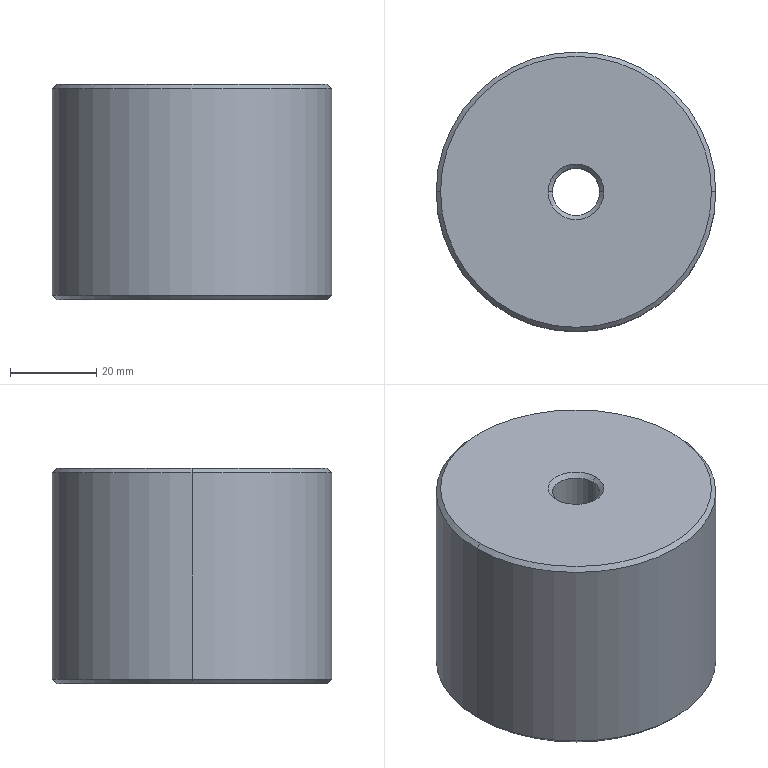Part | SolidWorks | features Chamfer 1, Extrusion 1 | 1 solid | 14 faces | box 65 x 65 x 50 mm | volume 160925 mm3 | cone 8 | cylinder 4 | plane 2 | commonest cylinder face diameters 11 x2 65 x2
STEP:
#1=CARTESIAN_POINT('',(31.5,0.,50.));
#2=VERTEX_POINT('',#1);
#3=CARTESIAN_POINT('',(-31.5,0.,50.));
#4=VERTEX_POINT('',#3);
#5=CARTESIAN_POINT('',(0.,0.,50.));
#6=DIRECTION('',(0.,0.,1.));
#7=DIRECTION('',(1.,0.,0.));
#8=AXIS2_PLACEMENT_3D('',#5,#6,#7);
#9=CIRCLE('',#8,31.5);
#10=EDGE_CURVE('',#2,#4,#9,.T.);
#11=ORIENTED_EDGE('',*,*,#10,.F.);
#12=CARTESIAN_POINT('',(32.5,0.,49.));
#13=VERTEX_POINT('',#12);
#14=CARTESIAN_POINT('',(31.5,0.,50.));
#15=DIRECTION('',(0.7071,0.,-0.7071));
#16=VECTOR('',#15,1000.);
#17=LINE('',#14,#16);
#18=EDGE_CURVE('',#2,#13,#17,.T.);
#19=ORIENTED_EDGE('',*,*,#18,.T.);
#20=CARTESIAN_POINT('',(-32.5,0.,49.));
#21=VERTEX_POINT('',#20);
#22=CARTESIAN_POINT('',(0.,0.,49.));
#23=DIRECTION('',(0.,0.,-1.));
#24=DIRECTION('',(1.,0.,0.));
#25=AXIS2_PLACEMENT_3D('',#22,#23,#24);
#26=CIRCLE('',#25,32.5);
#27=EDGE_CURVE('',#21,#13,#26,.T.);
#28=ORIENTED_EDGE('',*,*,#27,.F.);
#29=CARTESIAN_POINT('',(-31.5,0.,50.));
#30=DIRECTION('',(-0.7071,0.,-0.7071));
#31=VECTOR('',#30,1000.);
#32=LINE('',#29,#31);
#33=EDGE_CURVE('',#4,#21,#32,.T.);
#34=ORIENTED_EDGE('',*,*,#33,.F.);
#35=EDGE_LOOP('',(#11,#19,#28,#34));
#36=FACE_OUTER_BOUND('',#35,.T.);
#37=CARTESIAN_POINT('',(0.,0.,50.));
#38=DIRECTION('',(0.,0.,-1.));
#39=DIRECTION('',(-1.,0.,0.));
#40=AXIS2_PLACEMENT_3D('',#37,#38,#39);
#41=CONICAL_SURFACE('',#40,31.5,0.7854);
#42=ADVANCED_FACE('',(#36),#41,.T.);
#43=CARTESIAN_POINT('',(-5.5,0.,49.));
#44=VERTEX_POINT('',#43);
#45=CARTESIAN_POINT('',(5.5,0.,49.));
#46=VERTEX_POINT('',#45);
#47=CARTESIAN_POINT('',(0.,0.,49.));
#48=DIRECTION('',(0.,0.,1.));
#49=DIRECTION('',(1.,0.,0.));
#50=AXIS2_PLACEMENT_3D('',#47,#48,#49);
#51=CIRCLE('',#50,5.5);
#52=EDGE_CURVE('',#44,#46,#51,.T.);
#53=ORIENTED_EDGE('',*,*,#52,.F.);
#54=CARTESIAN_POINT('',(-6.5,0.,50.));
#55=VERTEX_POINT('',#54);
#56=CARTESIAN_POINT('',(-5.5,0.,49.));
#57=DIRECTION('',(-0.7071,0.,0.7071));
#58=VECTOR('',#57,1000.);
#59=LINE('',#56,#58);
#60=EDGE_CURVE('',#44,#55,#59,.T.);
#61=ORIENTED_EDGE('',*,*,#60,.T.);
#62=CARTESIAN_POINT('',(6.5,0.,50.));
#63=VERTEX_POINT('',#62);
#64=CARTESIAN_POINT('',(0.,0.,50.));
#65=DIRECTION('',(0.,0.,-1.));
#66=DIRECTION('',(1.,0.,0.));
#67=AXIS2_PLACEMENT_3D('',#64,#65,#66);
#68=CIRCLE('',#67,6.5);
#69=EDGE_CURVE('',#63,#55,#68,.T.);
#70=ORIENTED_EDGE('',*,*,#69,.F.);
#71=CARTESIAN_POINT('',(5.5,0.,49.));
#72=DIRECTION('',(0.7071,0.,0.7071));
#73=VECTOR('',#72,1000.);
#74=LINE('',#71,#73);
#75=EDGE_CURVE('',#46,#63,#74,.T.);
#76=ORIENTED_EDGE('',*,*,#75,.F.);
#77=EDGE_LOOP('',(#53,#61,#70,#76));
#78=FACE_OUTER_BOUND('',#77,.T.);
#79=CARTESIAN_POINT('',(0.,0.,49.));
#80=DIRECTION('',(0.,0.,1.));
#81=DIRECTION('',(1.,0.,0.));
#82=AXIS2_PLACEMENT_3D('',#79,#80,#81);
#83=CONICAL_SURFACE('',#82,5.5,0.7854);
#84=ADVANCED_FACE('',(#78),#83,.F.);
#85=CARTESIAN_POINT('',(-31.5,0.,0.));
#86=VERTEX_POINT('',#85);
#87=CARTESIAN_POINT('',(31.5,0.,0.));
#88=VERTEX_POINT('',#87);
#89=CARTESIAN_POINT('',(0.,0.,0.));
#90=DIRECTION('',(0.,0.,-1.));
#91=DIRECTION('',(1.,0.,0.));
#92=AXIS2_PLACEMENT_3D('',#89,#90,#91);
#93=CIRCLE('',#92,31.5);
#94=EDGE_CURVE('',#86,#88,#93,.T.);
#95=ORIENTED_EDGE('',*,*,#94,.F.);
#96=CARTESIAN_POINT('',(-32.5,0.,1.));
#97=VERTEX_POINT('',#96);
#98=CARTESIAN_POINT('',(-32.5,0.,1.));
#99=DIRECTION('',(-0.7071,0.,0.7071));
#100=VECTOR('',#99,1000.);
#101=LINE('',#98,#100);
#102=EDGE_CURVE('',#86,#97,#101,.T.);
#103=ORIENTED_EDGE('',*,*,#102,.T.);
#104=CARTESIAN_POINT('',(32.5,0.,1.));
#105=VERTEX_POINT('',#104);
#106=CARTESIAN_POINT('',(0.,0.,1.));
#107=DIRECTION('',(0.,0.,1.));
#108=DIRECTION('',(1.,0.,0.));
#109=AXIS2_PLACEMENT_3D('',#106,#107,#108);
#110=CIRCLE('',#109,32.5);
#111=EDGE_CURVE('',#105,#97,#110,.T.);
#112=ORIENTED_EDGE('',*,*,#111,.F.);
#113=CARTESIAN_POINT('',(32.5,0.,1.));
#114=DIRECTION('',(0.7071,0.,0.7071));
#115=VECTOR('',#114,1000.);
#116=LINE('',#113,#115);
#117=EDGE_CURVE('',#88,#105,#116,.T.);
#118=ORIENTED_EDGE('',*,*,#117,.F.);
#119=EDGE_LOOP('',(#95,#103,#112,#118));
#120=FACE_OUTER_BOUND('',#119,.T.);
#121=CARTESIAN_POINT('',(0.,0.,1.));
#122=DIRECTION('',(0.,0.,1.));
#123=DIRECTION('',(1.,0.,0.));
#124=AXIS2_PLACEMENT_3D('',#121,#122,#123);
#125=CONICAL_SURFACE('',#124,32.5,0.7854);
#126=ADVANCED_FACE('',(#120),#125,.T.);
#127=CARTESIAN_POINT('',(5.5,0.,1.));
#128=VERTEX_POINT('',#127);
#129=CARTESIAN_POINT('',(-5.5,0.,1.));
#130=VERTEX_POINT('',#129);
#131=CARTESIAN_POINT('',(0.,0.,1.));
#132=DIRECTION('',(0.,0.,-1.));
#133=DIRECTION('',(1.,0.,0.));
#134=AXIS2_PLACEMENT_3D('',#131,#132,#133);
#135=CIRCLE('',#134,5.5);
#136=EDGE_CURVE('',#128,#130,#135,.T.);
#137=ORIENTED_EDGE('',*,*,#136,.F.);
#138=CARTESIAN_POINT('',(6.5,0.,0.));
#139=VERTEX_POINT('',#138);
#140=CARTESIAN_POINT('',(6.5,0.,0.));
#141=DIRECTION('',(0.7071,0.,-0.7071));
#142=VECTOR('',#141,1000.);
#143=LINE('',#140,#142);
#144=EDGE_CURVE('',#128,#139,#143,.T.);
#145=ORIENTED_EDGE('',*,*,#144,.T.);
#146=CARTESIAN_POINT('',(-6.5,0.,0.));
#147=VERTEX_POINT('',#146);
#148=CARTESIAN_POINT('',(0.,0.,0.));
#149=DIRECTION('',(0.,0.,1.));
#150=DIRECTION('',(1.,0.,0.));
#151=AXIS2_PLACEMENT_3D('',#148,#149,#150);
#152=CIRCLE('',#151,6.5);
#153=EDGE_CURVE('',#147,#139,#152,.T.);
#154=ORIENTED_EDGE('',*,*,#153,.F.);
#155=CARTESIAN_POINT('',(-6.5,0.,0.));
#156=DIRECTION('',(-0.7071,0.,-0.7071));
#157=VECTOR('',#156,1000.);
#158=LINE('',#155,#157);
#159=EDGE_CURVE('',#130,#147,#158,.T.);
#160=ORIENTED_EDGE('',*,*,#159,.F.);
#161=EDGE_LOOP('',(#137,#145,#154,#160));
#162=FACE_OUTER_BOUND('',#161,.T.);
#163=CARTESIAN_POINT('',(0.,0.,0.));
#164=DIRECTION('',(0.,0.,-1.));
#165=DIRECTION('',(-1.,0.,0.));
#166=AXIS2_PLACEMENT_3D('',#163,#164,#165);
#167=CONICAL_SURFACE('',#166,6.5,0.7854);
#168=ADVANCED_FACE('',(#162),#167,.F.);
#169=ORIENTED_EDGE('',*,*,#52,.T.);
#170=CARTESIAN_POINT('',(5.5,0.,50.));
#171=DIRECTION('',(0.,0.,-1.));
#172=VECTOR('',#171,1000.);
#173=LINE('',#170,#172);
#174=EDGE_CURVE('',#46,#128,#173,.T.);
#175=ORIENTED_EDGE('',*,*,#174,.T.);
#176=ORIENTED_EDGE('',*,*,#136,.T.);
#177=CARTESIAN_POINT('',(-5.5,0.,50.));
#178=DIRECTION('',(0.,0.,-1.));
#179=VECTOR('',#178,1000.);
#180=LINE('',#177,#179);
#181=EDGE_CURVE('',#44,#130,#180,.T.);
#182=ORIENTED_EDGE('',*,*,#181,.F.);
#183=EDGE_LOOP('',(#169,#175,#176,#182));
#184=FACE_OUTER_BOUND('',#183,.T.);
#185=CARTESIAN_POINT('',(0.,0.,50.));
#186=DIRECTION('',(0.,0.,-1.));
#187=DIRECTION('',(-1.,0.,0.));
#188=AXIS2_PLACEMENT_3D('',#185,#186,#187);
#189=CYLINDRICAL_SURFACE('',#188,5.5);
#190=ADVANCED_FACE('',(#184),#189,.F.);
#191=ORIENTED_EDGE('',*,*,#27,.T.);
#192=CARTESIAN_POINT('',(32.5,0.,50.));
#193=DIRECTION('',(0.,0.,-1.));
#194=VECTOR('',#193,1000.);
#195=LINE('',#192,#194);
#196=EDGE_CURVE('',#13,#105,#195,.T.);
#197=ORIENTED_EDGE('',*,*,#196,.T.);
#198=ORIENTED_EDGE('',*,*,#111,.T.);
#199=CARTESIAN_POINT('',(-32.5,0.,50.));
#200=DIRECTION('',(0.,0.,-1.));
#201=VECTOR('',#200,1000.);
#202=LINE('',#199,#201);
#203=EDGE_CURVE('',#21,#97,#202,.T.);
#204=ORIENTED_EDGE('',*,*,#203,.F.);
#205=EDGE_LOOP('',(#191,#197,#198,#204));
#206=FACE_OUTER_BOUND('',#205,.T.);
#207=CARTESIAN_POINT('',(0.,0.,50.));
#208=DIRECTION('',(0.,0.,-1.));
#209=DIRECTION('',(-1.,0.,0.));
#210=AXIS2_PLACEMENT_3D('',#207,#208,#209);
#211=CYLINDRICAL_SURFACE('',#210,32.5);
#212=ADVANCED_FACE('',(#206),#211,.T.);
#213=ORIENTED_EDGE('',*,*,#69,.T.);
#214=CARTESIAN_POINT('',(0.,0.,50.));
#215=DIRECTION('',(0.,0.,-1.));
#216=DIRECTION('',(1.,0.,0.));
#217=AXIS2_PLACEMENT_3D('',#214,#215,#216);
#218=CIRCLE('',#217,6.5);
#219=EDGE_CURVE('',#55,#63,#218,.T.);
#220=ORIENTED_EDGE('',*,*,#219,.T.);
#221=EDGE_LOOP('',(#213,#220));
#222=FACE_BOUND('',#221,.T.);
#223=CARTESIAN_POINT('',(0.,0.,50.));
#224=DIRECTION('',(0.,0.,1.));
#225=DIRECTION('',(1.,0.,0.));
#226=AXIS2_PLACEMENT_3D('',#223,#224,#225);
#227=CIRCLE('',#226,31.5);
#228=EDGE_CURVE('',#4,#2,#227,.T.);
#229=ORIENTED_EDGE('',*,*,#228,.T.);
#230=ORIENTED_EDGE('',*,*,#10,.T.);
#231=EDGE_LOOP('',(#229,#230));
#232=FACE_OUTER_BOUND('',#231,.T.);
#233=CARTESIAN_POINT('',(0.,0.,50.));
#234=DIRECTION('',(0.,0.,1.));
#235=DIRECTION('',(1.,0.,0.));
#236=AXIS2_PLACEMENT_3D('',#233,#234,#235);
#237=PLANE('',#236);
#238=ADVANCED_FACE('',(#222,#232),#237,.T.);
#239=ORIENTED_EDGE('',*,*,#153,.T.);
#240=CARTESIAN_POINT('',(0.,0.,0.));
#241=DIRECTION('',(0.,0.,1.));
#242=DIRECTION('',(1.,0.,0.));
#243=AXIS2_PLACEMENT_3D('',#240,#241,#242);
#244=CIRCLE('',#243,6.5);
#245=EDGE_CURVE('',#139,#147,#244,.T.);
#246=ORIENTED_EDGE('',*,*,#245,.T.);
#247=EDGE_LOOP('',(#239,#246));
#248=FACE_BOUND('',#247,.T.);
#249=CARTESIAN_POINT('',(0.,0.,0.));
#250=DIRECTION('',(0.,0.,-1.));
#251=DIRECTION('',(1.,0.,0.));
#252=AXIS2_PLACEMENT_3D('',#249,#250,#251);
#253=CIRCLE('',#252,31.5);
#254=EDGE_CURVE('',#88,#86,#253,.T.);
#255=ORIENTED_EDGE('',*,*,#254,.T.);
#256=ORIENTED_EDGE('',*,*,#94,.T.);
#257=EDGE_LOOP('',(#255,#256));
#258=FACE_OUTER_BOUND('',#257,.T.);
#259=CARTESIAN_POINT('',(0.,0.,0.));
#260=DIRECTION('',(0.,0.,1.));
#261=DIRECTION('',(1.,0.,0.));
#262=AXIS2_PLACEMENT_3D('',#259,#260,#261);
#263=PLANE('',#262);
#264=ADVANCED_FACE('',(#248,#258),#263,.F.);
#265=ORIENTED_EDGE('',*,*,#196,.F.);
#266=CARTESIAN_POINT('',(0.,0.,49.));
#267=DIRECTION('',(0.,0.,-1.));
#268=DIRECTION('',(1.,0.,0.));
#269=AXIS2_PLACEMENT_3D('',#266,#267,#268);
#270=CIRCLE('',#269,32.5);
#271=EDGE_CURVE('',#13,#21,#270,.T.);
#272=ORIENTED_EDGE('',*,*,#271,.T.);
#273=ORIENTED_EDGE('',*,*,#203,.T.);
#274=CARTESIAN_POINT('',(0.,0.,1.));
#275=DIRECTION('',(0.,0.,1.));
#276=DIRECTION('',(1.,0.,0.));
#277=AXIS2_PLACEMENT_3D('',#274,#275,#276);
#278=CIRCLE('',#277,32.5);
#279=EDGE_CURVE('',#97,#105,#278,.T.);
#280=ORIENTED_EDGE('',*,*,#279,.T.);
#281=EDGE_LOOP('',(#265,#272,#273,#280));
#282=FACE_OUTER_BOUND('',#281,.T.);
#283=CARTESIAN_POINT('',(0.,0.,50.));
#284=DIRECTION('',(0.,0.,-1.));
#285=DIRECTION('',(-1.,0.,0.));
#286=AXIS2_PLACEMENT_3D('',#283,#284,#285);
#287=CYLINDRICAL_SURFACE('',#286,32.5);
#288=ADVANCED_FACE('',(#282),#287,.T.);
#289=ORIENTED_EDGE('',*,*,#174,.F.);
#290=CARTESIAN_POINT('',(0.,0.,49.));
#291=DIRECTION('',(0.,0.,1.));
#292=DIRECTION('',(1.,0.,0.));
#293=AXIS2_PLACEMENT_3D('',#290,#291,#292);
#294=CIRCLE('',#293,5.5);
#295=EDGE_CURVE('',#46,#44,#294,.T.);
#296=ORIENTED_EDGE('',*,*,#295,.T.);
#297=ORIENTED_EDGE('',*,*,#181,.T.);
#298=CARTESIAN_POINT('',(0.,0.,1.));
#299=DIRECTION('',(0.,0.,-1.));
#300=DIRECTION('',(1.,0.,0.));
#301=AXIS2_PLACEMENT_3D('',#298,#299,#300);
#302=CIRCLE('',#301,5.5);
#303=EDGE_CURVE('',#130,#128,#302,.T.);
#304=ORIENTED_EDGE('',*,*,#303,.T.);
#305=EDGE_LOOP('',(#289,#296,#297,#304));
#306=FACE_OUTER_BOUND('',#305,.T.);
#307=CARTESIAN_POINT('',(0.,0.,50.));
#308=DIRECTION('',(0.,0.,-1.));
#309=DIRECTION('',(-1.,0.,0.));
#310=AXIS2_PLACEMENT_3D('',#307,#308,#309);
#311=CYLINDRICAL_SURFACE('',#310,5.5);
#312=ADVANCED_FACE('',(#306),#311,.F.);
#313=ORIENTED_EDGE('',*,*,#144,.F.);
#314=ORIENTED_EDGE('',*,*,#303,.F.);
#315=ORIENTED_EDGE('',*,*,#159,.T.);
#316=ORIENTED_EDGE('',*,*,#245,.F.);
#317=EDGE_LOOP('',(#313,#314,#315,#316));
#318=FACE_OUTER_BOUND('',#317,.T.);
#319=CARTESIAN_POINT('',(0.,0.,0.));
#320=DIRECTION('',(0.,0.,-1.));
#321=DIRECTION('',(-1.,0.,0.));
#322=AXIS2_PLACEMENT_3D('',#319,#320,#321);
#323=CONICAL_SURFACE('',#322,6.5,0.7854);
#324=ADVANCED_FACE('',(#318),#323,.F.);
#325=ORIENTED_EDGE('',*,*,#102,.F.);
#326=ORIENTED_EDGE('',*,*,#254,.F.);
#327=ORIENTED_EDGE('',*,*,#117,.T.);
#328=ORIENTED_EDGE('',*,*,#279,.F.);
#329=EDGE_LOOP('',(#325,#326,#327,#328));
#330=FACE_OUTER_BOUND('',#329,.T.);
#331=CARTESIAN_POINT('',(0.,0.,1.));
#332=DIRECTION('',(0.,0.,1.));
#333=DIRECTION('',(1.,0.,0.));
#334=AXIS2_PLACEMENT_3D('',#331,#332,#333);
#335=CONICAL_SURFACE('',#334,32.5,0.7854);
#336=ADVANCED_FACE('',(#330),#335,.T.);
#337=ORIENTED_EDGE('',*,*,#60,.F.);
#338=ORIENTED_EDGE('',*,*,#295,.F.);
#339=ORIENTED_EDGE('',*,*,#75,.T.);
#340=ORIENTED_EDGE('',*,*,#219,.F.);
#341=EDGE_LOOP('',(#337,#338,#339,#340));
#342=FACE_OUTER_BOUND('',#341,.T.);
#343=CARTESIAN_POINT('',(0.,0.,49.));
#344=DIRECTION('',(0.,0.,1.));
#345=DIRECTION('',(1.,0.,0.));
#346=AXIS2_PLACEMENT_3D('',#343,#344,#345);
#347=CONICAL_SURFACE('',#346,5.5,0.7854);
#348=ADVANCED_FACE('',(#342),#347,.F.);
#349=ORIENTED_EDGE('',*,*,#18,.F.);
#350=ORIENTED_EDGE('',*,*,#228,.F.);
#351=ORIENTED_EDGE('',*,*,#33,.T.);
#352=ORIENTED_EDGE('',*,*,#271,.F.);
#353=EDGE_LOOP('',(#349,#350,#351,#352));
#354=FACE_OUTER_BOUND('',#353,.T.);
#355=CARTESIAN_POINT('',(0.,0.,50.));
#356=DIRECTION('',(0.,0.,-1.));
#357=DIRECTION('',(-1.,0.,0.));
#358=AXIS2_PLACEMENT_3D('',#355,#356,#357);
#359=CONICAL_SURFACE('',#358,31.5,0.7854);
#360=ADVANCED_FACE('',(#354),#359,.T.);
#361=CLOSED_SHELL('',(#42,#84,#126,#168,#190,#212,#238,#264,#288,#312,#324,#336,#348,#360));
#362=MANIFOLD_SOLID_BREP('',#361);
#363=CARTESIAN_POINT('',(0.,0.,0.));
#364=DIRECTION('',(0.,0.,1.));
#365=DIRECTION('',(1.,0.,0.));
#366=AXIS2_PLACEMENT_3D('',#363,#364,#365);
#367=(LENGTH_UNIT()NAMED_UNIT(*)SI_UNIT(.MILLI.,.METRE.));
#368=UNCERTAINTY_MEASURE_WITH_UNIT(LENGTH_MEASURE(0.00001),#367,'','');
#369=(NAMED_UNIT(*)PLANE_ANGLE_UNIT()SI_UNIT($,.RADIAN.));
#370=(NAMED_UNIT(*)SI_UNIT($,.STERADIAN.)SOLID_ANGLE_UNIT());
#371=(GEOMETRIC_REPRESENTATION_CONTEXT(3)GLOBAL_UNCERTAINTY_ASSIGNED_CONTEXT((#368))GLOBAL_UNIT_ASSIGNED_CONTEXT((#367,#369,#370))REPRESENTATION_CONTEXT('',''));
#372=ADVANCED_BREP_SHAPE_REPRESENTATION('',(#362,#366),#371);